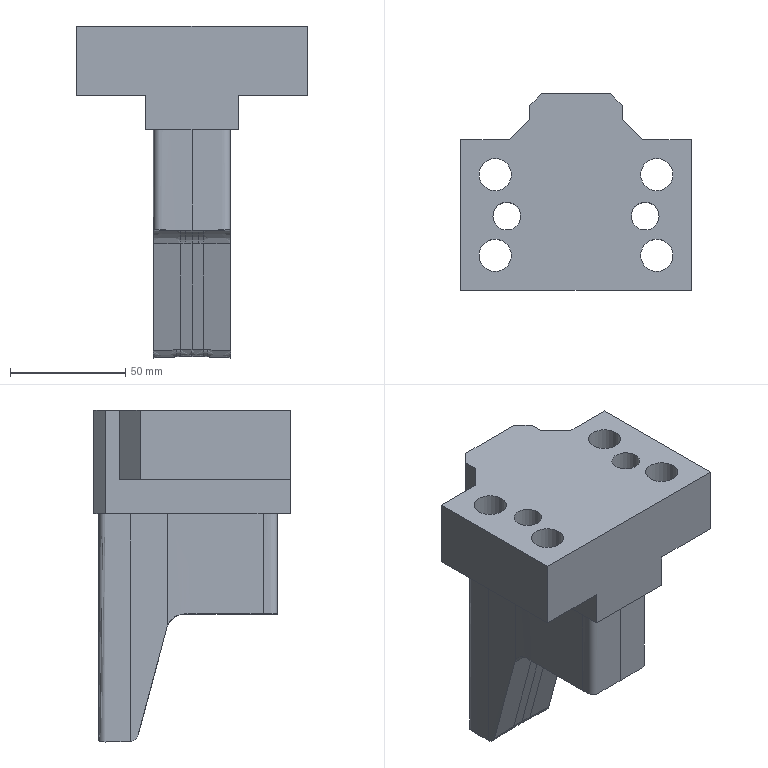Part | NX | features solid 2 | 1 solid | 61 faces | box 100 x 85 x 143.799 mm | volume 391184 mm3 | spline 29 | plane 22 | cylinder 10 | commonest cylinder face diameters 14 x4 20 x4 12 x2